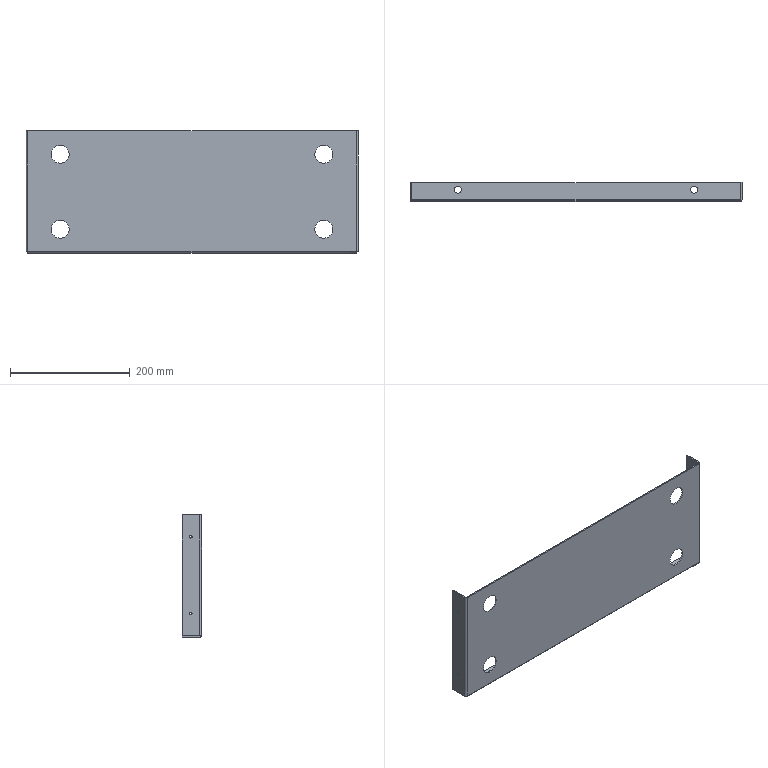Part | NX | 1 solid | 40 faces | box 554 x 32 x 204 mm | volume 275218 mm3 | plane 20 | cylinder 16 | spline 4 | commonest cylinder face diameters 4.2 x4 30 x4 2 x3 6 x3 12 x2
STEP:
#1=CARTESIAN_POINT('',(-274.293,30.,-103.));
#2=VERTEX_POINT('',#1);
#3=CARTESIAN_POINT('',(-274.293,1.,-103.));
#4=VERTEX_POINT('',#3);
#5=CARTESIAN_POINT('',(-274.293,0.,-103.));
#6=DIRECTION('',(0.,-1.,0.));
#7=VECTOR('',#6,1000.);
#8=LINE('',#5,#7);
#9=EDGE_CURVE('',#2,#4,#8,.T.);
#10=ORIENTED_EDGE('',*,*,#9,.F.);
#11=CARTESIAN_POINT('',(274.293,30.,-103.));
#12=VERTEX_POINT('',#11);
#13=CARTESIAN_POINT('',(-275.,30.,-103.));
#14=DIRECTION('',(1.,0.,0.));
#15=VECTOR('',#14,1000.);
#16=LINE('',#13,#15);
#17=EDGE_CURVE('',#2,#12,#16,.T.);
#18=ORIENTED_EDGE('',*,*,#17,.T.);
#19=CARTESIAN_POINT('',(274.293,1.,-103.));
#20=VERTEX_POINT('',#19);
#21=CARTESIAN_POINT('',(274.293,0.,-103.));
#22=DIRECTION('',(0.,-1.,0.));
#23=VECTOR('',#22,1000.);
#24=LINE('',#21,#23);
#25=EDGE_CURVE('',#12,#20,#24,.T.);
#26=ORIENTED_EDGE('',*,*,#25,.T.);
#27=CARTESIAN_POINT('',(0.,1.,-103.));
#28=DIRECTION('',(-1.,0.,0.));
#29=VECTOR('',#28,1000.);
#30=LINE('',#27,#29);
#31=EDGE_CURVE('',#20,#4,#30,.T.);
#32=ORIENTED_EDGE('',*,*,#31,.T.);
#33=EDGE_LOOP('',(#10,#18,#26,#32));
#34=FACE_BOUND('',#33,.T.);
#35=CARTESIAN_POINT('',(-197.,24.,-103.));
#36=VERTEX_POINT('',#35);
#37=CARTESIAN_POINT('',(-197.,18.,-103.));
#38=DIRECTION('',(0.,0.,-1.));
#39=DIRECTION('',(0.,1.,0.));
#40=AXIS2_PLACEMENT_3D('',#37,#38,#39);
#41=CIRCLE('',#40,6.);
#42=EDGE_CURVE('',#36,#36,#41,.T.);
#43=ORIENTED_EDGE('',*,*,#42,.F.);
#44=EDGE_LOOP('',(#43));
#45=FACE_BOUND('',#44,.T.);
#46=CARTESIAN_POINT('',(197.,24.,-103.));
#47=VERTEX_POINT('',#46);
#48=CARTESIAN_POINT('',(197.,18.,-103.));
#49=DIRECTION('',(0.,0.,1.));
#50=DIRECTION('',(0.,1.,0.));
#51=AXIS2_PLACEMENT_3D('',#48,#49,#50);
#52=CIRCLE('',#51,6.);
#53=EDGE_CURVE('',#47,#47,#52,.T.);
#54=ORIENTED_EDGE('',*,*,#53,.T.);
#55=EDGE_LOOP('',(#54));
#56=FACE_BOUND('',#55,.T.);
#57=CARTESIAN_POINT('',(0.,0.,-103.));
#58=DIRECTION('',(0.,0.,-1.));
#59=DIRECTION('',(0.,1.,0.));
#60=AXIS2_PLACEMENT_3D('',#57,#58,#59);
#61=PLANE('',#60);
#62=ADVANCED_FACE('',(#34,#45,#56),#61,.T.);
#63=CARTESIAN_POINT('',(-274.293,30.,-101.));
#64=VERTEX_POINT('',#63);
#65=CARTESIAN_POINT('',(274.293,30.,-101.));
#66=VERTEX_POINT('',#65);
#67=CARTESIAN_POINT('',(-275.,30.,-101.));
#68=DIRECTION('',(1.,0.,0.));
#69=VECTOR('',#68,1000.);
#70=LINE('',#67,#69);
#71=EDGE_CURVE('',#64,#66,#70,.T.);
#72=ORIENTED_EDGE('',*,*,#71,.F.);
#73=CARTESIAN_POINT('',(-274.293,1.,-101.));
#74=VERTEX_POINT('',#73);
#75=CARTESIAN_POINT('',(-274.293,0.,-101.));
#76=DIRECTION('',(0.,1.,0.));
#77=VECTOR('',#76,1000.);
#78=LINE('',#75,#77);
#79=EDGE_CURVE('',#74,#64,#78,.T.);
#80=ORIENTED_EDGE('',*,*,#79,.F.);
#81=CARTESIAN_POINT('',(274.293,1.,-101.));
#82=VERTEX_POINT('',#81);
#83=CARTESIAN_POINT('',(275.,1.,-101.));
#84=DIRECTION('',(-1.,0.,0.));
#85=VECTOR('',#84,1000.);
#86=LINE('',#83,#85);
#87=EDGE_CURVE('',#82,#74,#86,.T.);
#88=ORIENTED_EDGE('',*,*,#87,.F.);
#89=CARTESIAN_POINT('',(274.293,0.,-101.));
#90=DIRECTION('',(0.,1.,0.));
#91=VECTOR('',#90,1000.);
#92=LINE('',#89,#91);
#93=EDGE_CURVE('',#82,#66,#92,.T.);
#94=ORIENTED_EDGE('',*,*,#93,.T.);
#95=EDGE_LOOP('',(#72,#80,#88,#94));
#96=FACE_BOUND('',#95,.T.);
#97=CARTESIAN_POINT('',(-197.,24.,-101.));
#98=VERTEX_POINT('',#97);
#99=CARTESIAN_POINT('',(-197.,18.,-101.));
#100=DIRECTION('',(0.,0.,-1.));
#101=DIRECTION('',(0.,1.,0.));
#102=AXIS2_PLACEMENT_3D('',#99,#100,#101);
#103=CIRCLE('',#102,6.);
#104=EDGE_CURVE('',#98,#98,#103,.F.);
#105=ORIENTED_EDGE('',*,*,#104,.F.);
#106=EDGE_LOOP('',(#105));
#107=FACE_BOUND('',#106,.T.);
#108=CARTESIAN_POINT('',(197.,24.,-101.));
#109=VERTEX_POINT('',#108);
#110=CARTESIAN_POINT('',(197.,18.,-101.));
#111=DIRECTION('',(0.,0.,-1.));
#112=DIRECTION('',(0.,1.,0.));
#113=AXIS2_PLACEMENT_3D('',#110,#111,#112);
#114=CIRCLE('',#113,6.);
#115=EDGE_CURVE('',#109,#109,#114,.T.);
#116=ORIENTED_EDGE('',*,*,#115,.T.);
#117=EDGE_LOOP('',(#116));
#118=FACE_BOUND('',#117,.T.);
#119=CARTESIAN_POINT('',(0.,0.,-101.));
#120=DIRECTION('',(0.,0.,-1.));
#121=DIRECTION('',(0.,1.,0.));
#122=AXIS2_PLACEMENT_3D('',#119,#120,#121);
#123=PLANE('',#122);
#124=ADVANCED_FACE('',(#96,#107,#118),#123,.F.);
#125=CARTESIAN_POINT('',(220.,-2.,-48.));
#126=VERTEX_POINT('',#125);
#127=CARTESIAN_POINT('',(220.,-2.,-63.));
#128=DIRECTION('',(0.,-1.,0.));
#129=DIRECTION('',(0.,0.,1.));
#130=AXIS2_PLACEMENT_3D('',#127,#128,#129);
#131=CIRCLE('',#130,15.);
#132=EDGE_CURVE('',#126,#126,#131,.T.);
#133=ORIENTED_EDGE('',*,*,#132,.F.);
#134=EDGE_LOOP('',(#133));
#135=FACE_BOUND('',#134,.T.);
#136=CARTESIAN_POINT('',(-220.,-2.,47.));
#137=VERTEX_POINT('',#136);
#138=CARTESIAN_POINT('',(-220.,-2.,62.));
#139=DIRECTION('',(0.,-1.,0.));
#140=DIRECTION('',(0.,0.,-1.));
#141=AXIS2_PLACEMENT_3D('',#138,#139,#140);
#142=CIRCLE('',#141,15.);
#143=EDGE_CURVE('',#137,#137,#142,.T.);
#144=ORIENTED_EDGE('',*,*,#143,.F.);
#145=EDGE_LOOP('',(#144));
#146=FACE_BOUND('',#145,.T.);
#147=CARTESIAN_POINT('',(-220.,-2.,-78.));
#148=VERTEX_POINT('',#147);
#149=CARTESIAN_POINT('',(-220.,-2.,-63.));
#150=DIRECTION('',(0.,-1.,0.));
#151=DIRECTION('',(0.,0.,-1.));
#152=AXIS2_PLACEMENT_3D('',#149,#150,#151);
#153=CIRCLE('',#152,15.);
#154=EDGE_CURVE('',#148,#148,#153,.T.);
#155=ORIENTED_EDGE('',*,*,#154,.F.);
#156=EDGE_LOOP('',(#155));
#157=FACE_BOUND('',#156,.T.);
#158=CARTESIAN_POINT('',(-274.,-2.,101.));
#159=VERTEX_POINT('',#158);
#160=CARTESIAN_POINT('',(-274.,-2.,-100.));
#161=VERTEX_POINT('',#160);
#162=CARTESIAN_POINT('',(-274.,-2.,101.));
#163=DIRECTION('',(0.,0.,1.));
#164=VECTOR('',#163,1000.);
#165=LINE('',#162,#164);
#166=EDGE_CURVE('',#159,#161,#165,.F.);
#167=ORIENTED_EDGE('',*,*,#166,.T.);
#168=CARTESIAN_POINT('',(274.,-2.,-100.));
#169=VERTEX_POINT('',#168);
#170=CARTESIAN_POINT('',(-274.293,-2.,-100.));
#171=DIRECTION('',(-1.,0.,0.));
#172=VECTOR('',#171,1000.);
#173=LINE('',#170,#172);
#174=EDGE_CURVE('',#161,#169,#173,.F.);
#175=ORIENTED_EDGE('',*,*,#174,.T.);
#176=CARTESIAN_POINT('',(274.,-2.,101.));
#177=VERTEX_POINT('',#176);
#178=CARTESIAN_POINT('',(274.,-2.,-100.293));
#179=DIRECTION('',(0.,0.,-1.));
#180=VECTOR('',#179,1000.);
#181=LINE('',#178,#180);
#182=EDGE_CURVE('',#169,#177,#181,.F.);
#183=ORIENTED_EDGE('',*,*,#182,.T.);
#184=CARTESIAN_POINT('',(-275.,-2.,101.));
#185=DIRECTION('',(1.,0.,0.));
#186=VECTOR('',#185,1000.);
#187=LINE('',#184,#186);
#188=EDGE_CURVE('',#159,#177,#187,.T.);
#189=ORIENTED_EDGE('',*,*,#188,.F.);
#190=EDGE_LOOP('',(#167,#175,#183,#189));
#191=FACE_BOUND('',#190,.T.);
#192=CARTESIAN_POINT('',(220.,-2.,77.));
#193=VERTEX_POINT('',#192);
#194=CARTESIAN_POINT('',(220.,-2.,62.));
#195=DIRECTION('',(0.,-1.,0.));
#196=DIRECTION('',(0.,0.,1.));
#197=AXIS2_PLACEMENT_3D('',#194,#195,#196);
#198=CIRCLE('',#197,15.);
#199=EDGE_CURVE('',#193,#193,#198,.T.);
#200=ORIENTED_EDGE('',*,*,#199,.F.);
#201=EDGE_LOOP('',(#200));
#202=FACE_BOUND('',#201,.T.);
#203=CARTESIAN_POINT('',(0.,-2.,0.));
#204=DIRECTION('',(0.,-1.,0.));
#205=DIRECTION('',(0.,0.,-1.));
#206=AXIS2_PLACEMENT_3D('',#203,#204,#205);
#207=PLANE('',#206);
#208=ADVANCED_FACE('',(#135,#146,#157,#191,#202),#207,.T.);
#209=CARTESIAN_POINT('',(220.,0.,-48.));
#210=VERTEX_POINT('',#209);
#211=CARTESIAN_POINT('',(220.,0.,-63.));
#212=DIRECTION('',(0.,-1.,0.));
#213=DIRECTION('',(0.,0.,1.));
#214=AXIS2_PLACEMENT_3D('',#211,#212,#213);
#215=CIRCLE('',#214,15.);
#216=EDGE_CURVE('',#210,#210,#215,.T.);
#217=ORIENTED_EDGE('',*,*,#216,.T.);
#218=EDGE_LOOP('',(#217));
#219=FACE_BOUND('',#218,.T.);
#220=CARTESIAN_POINT('',(-220.,0.,77.));
#221=VERTEX_POINT('',#220);
#222=CARTESIAN_POINT('',(-220.,0.,62.));
#223=DIRECTION('',(0.,1.,0.));
#224=DIRECTION('',(0.,0.,1.));
#225=AXIS2_PLACEMENT_3D('',#222,#223,#224);
#226=CIRCLE('',#225,15.);
#227=EDGE_CURVE('',#221,#221,#226,.T.);
#228=ORIENTED_EDGE('',*,*,#227,.F.);
#229=EDGE_LOOP('',(#228));
#230=FACE_BOUND('',#229,.T.);
#231=CARTESIAN_POINT('',(-220.,0.,-48.));
#232=VERTEX_POINT('',#231);
#233=CARTESIAN_POINT('',(-220.,0.,-63.));
#234=DIRECTION('',(0.,1.,0.));
#235=DIRECTION('',(0.,0.,1.));
#236=AXIS2_PLACEMENT_3D('',#233,#234,#235);
#237=CIRCLE('',#236,15.);
#238=EDGE_CURVE('',#232,#232,#237,.T.);
#239=ORIENTED_EDGE('',*,*,#238,.F.);
#240=EDGE_LOOP('',(#239));
#241=FACE_BOUND('',#240,.T.);
#242=CARTESIAN_POINT('',(-274.,0.,-100.));
#243=VERTEX_POINT('',#242);
#244=CARTESIAN_POINT('',(274.,0.,-100.));
#245=VERTEX_POINT('',#244);
#246=CARTESIAN_POINT('',(-274.293,0.,-100.));
#247=DIRECTION('',(-1.,0.,0.));
#248=VECTOR('',#247,1000.);
#249=LINE('',#246,#248);
#250=EDGE_CURVE('',#243,#245,#249,.F.);
#251=ORIENTED_EDGE('',*,*,#250,.F.);
#252=CARTESIAN_POINT('',(-274.,0.,101.));
#253=VERTEX_POINT('',#252);
#254=CARTESIAN_POINT('',(-274.,0.,101.));
#255=DIRECTION('',(0.,0.,1.));
#256=VECTOR('',#255,1000.);
#257=LINE('',#254,#256);
#258=EDGE_CURVE('',#253,#243,#257,.F.);
#259=ORIENTED_EDGE('',*,*,#258,.F.);
#260=CARTESIAN_POINT('',(274.,0.,101.));
#261=VERTEX_POINT('',#260);
#262=CARTESIAN_POINT('',(-275.,0.,101.));
#263=DIRECTION('',(1.,0.,0.));
#264=VECTOR('',#263,1000.);
#265=LINE('',#262,#264);
#266=EDGE_CURVE('',#253,#261,#265,.T.);
#267=ORIENTED_EDGE('',*,*,#266,.T.);
#268=CARTESIAN_POINT('',(274.,0.,-100.293));
#269=DIRECTION('',(0.,0.,-1.));
#270=VECTOR('',#269,1000.);
#271=LINE('',#268,#270);
#272=EDGE_CURVE('',#245,#261,#271,.F.);
#273=ORIENTED_EDGE('',*,*,#272,.F.);
#274=EDGE_LOOP('',(#251,#259,#267,#273));
#275=FACE_BOUND('',#274,.T.);
#276=CARTESIAN_POINT('',(220.,0.,77.));
#277=VERTEX_POINT('',#276);
#278=CARTESIAN_POINT('',(220.,0.,62.));
#279=DIRECTION('',(0.,-1.,0.));
#280=DIRECTION('',(0.,0.,1.));
#281=AXIS2_PLACEMENT_3D('',#278,#279,#280);
#282=CIRCLE('',#281,15.);
#283=EDGE_CURVE('',#277,#277,#282,.T.);
#284=ORIENTED_EDGE('',*,*,#283,.T.);
#285=EDGE_LOOP('',(#284));
#286=FACE_BOUND('',#285,.T.);
#287=CARTESIAN_POINT('',(0.,0.,0.));
#288=DIRECTION('',(0.,-1.,0.));
#289=DIRECTION('',(0.,0.,-1.));
#290=AXIS2_PLACEMENT_3D('',#287,#288,#289);
#291=PLANE('',#290);
#292=ADVANCED_FACE('',(#219,#230,#241,#275,#286),#291,.F.);
#293=ORIENTED_EDGE('',*,*,#266,.F.);
#294=CARTESIAN_POINT('',(-274.,0.,101.));
#295=DIRECTION('',(0.,-1.,0.));
#296=VECTOR('',#295,1000.);
#297=LINE('',#294,#296);
#298=EDGE_CURVE('',#253,#159,#297,.T.);
#299=ORIENTED_EDGE('',*,*,#298,.T.);
#300=ORIENTED_EDGE('',*,*,#188,.T.);
#301=CARTESIAN_POINT('',(274.,0.,101.));
#302=DIRECTION('',(0.,-1.,0.));
#303=VECTOR('',#302,1000.);
#304=LINE('',#301,#303);
#305=EDGE_CURVE('',#261,#177,#304,.T.);
#306=ORIENTED_EDGE('',*,*,#305,.F.);
#307=EDGE_LOOP('',(#293,#299,#300,#306));
#308=FACE_BOUND('',#307,.T.);
#309=CARTESIAN_POINT('',(-275.,-2.,101.));
#310=DIRECTION('',(0.,0.,1.));
#311=DIRECTION('',(1.,0.,0.));
#312=AXIS2_PLACEMENT_3D('',#309,#310,#311);
#313=PLANE('',#312);
#314=ADVANCED_FACE('',(#308),#313,.T.);
#315=CARTESIAN_POINT('',(275.,1.,101.));
#316=VERTEX_POINT('',#315);
#317=CARTESIAN_POINT('',(277.,1.,101.));
#318=VERTEX_POINT('',#317);
#319=CARTESIAN_POINT('',(275.,1.,101.));
#320=DIRECTION('',(1.,0.,0.));
#321=VECTOR('',#320,1000.);
#322=LINE('',#319,#321);
#323=EDGE_CURVE('',#316,#318,#322,.T.);
#324=ORIENTED_EDGE('',*,*,#323,.F.);
#325=CARTESIAN_POINT('',(274.,1.,101.));
#326=DIRECTION('',(0.,0.,-1.));
#327=DIRECTION('',(-1.,0.,0.));
#328=AXIS2_PLACEMENT_3D('',#325,#326,#327);
#329=CIRCLE('',#328,1.);
#330=EDGE_CURVE('',#261,#316,#329,.F.);
#331=ORIENTED_EDGE('',*,*,#330,.F.);
#332=ORIENTED_EDGE('',*,*,#305,.T.);
#333=CARTESIAN_POINT('',(274.,1.,101.));
#334=DIRECTION('',(0.,0.,-1.));
#335=DIRECTION('',(-1.,0.,0.));
#336=AXIS2_PLACEMENT_3D('',#333,#334,#335);
#337=CIRCLE('',#336,3.);
#338=EDGE_CURVE('',#177,#318,#337,.F.);
#339=ORIENTED_EDGE('',*,*,#338,.T.);
#340=EDGE_LOOP('',(#324,#331,#332,#339));
#341=FACE_BOUND('',#340,.T.);
#342=CARTESIAN_POINT('',(274.,1.,101.));
#343=DIRECTION('',(0.,0.,1.));
#344=DIRECTION('',(1.,0.,0.));
#345=AXIS2_PLACEMENT_3D('',#342,#343,#344);
#346=PLANE('',#345);
#347=ADVANCED_FACE('',(#341),#346,.T.);
#348=CARTESIAN_POINT('',(275.,1.,-100.293));
#349=VERTEX_POINT('',#348);
#350=CARTESIAN_POINT('',(275.,1.,-100.293));
#351=CARTESIAN_POINT('',(275.,0.4764,-100.195));
#352=CARTESIAN_POINT('',(274.524,0.,-100.098));
#353=CARTESIAN_POINT('',(274.,0.,-100.));
#354=B_SPLINE_CURVE_WITH_KNOTS('',3,(#350,#351,#352,#353),.UNSPECIFIED.,.F.,.F.,(4,4),(0.,1.),.UNSPECIFIED.);
#355=EDGE_CURVE('',#349,#245,#354,.T.);
#356=ORIENTED_EDGE('',*,*,#355,.F.);
#357=CARTESIAN_POINT('',(277.,1.,-100.293));
#358=VERTEX_POINT('',#357);
#359=CARTESIAN_POINT('',(275.,1.,-100.293));
#360=DIRECTION('',(-1.,0.,0.));
#361=VECTOR('',#360,1000.);
#362=LINE('',#359,#361);
#363=EDGE_CURVE('',#358,#349,#362,.T.);
#364=ORIENTED_EDGE('',*,*,#363,.F.);
#365=CARTESIAN_POINT('',(277.,1.,-100.293));
#366=CARTESIAN_POINT('',(277.,0.2146,-100.244));
#367=CARTESIAN_POINT('',(276.35,-1.35,-100.146));
#368=CARTESIAN_POINT('',(274.785,-2.,-100.049));
#369=CARTESIAN_POINT('',(274.,-2.,-100.));
#370=B_SPLINE_CURVE_WITH_KNOTS('',3,(#365,#366,#367,#368,#369),.UNSPECIFIED.,.F.,.F.,(4,1,4),(0.,0.5,1.),.UNSPECIFIED.);
#371=EDGE_CURVE('',#358,#169,#370,.T.);
#372=ORIENTED_EDGE('',*,*,#371,.T.);
#373=CARTESIAN_POINT('',(274.,0.,-100.));
#374=DIRECTION('',(0.,-1.,0.));
#375=VECTOR('',#374,1000.);
#376=LINE('',#373,#375);
#377=EDGE_CURVE('',#245,#169,#376,.T.);
#378=ORIENTED_EDGE('',*,*,#377,.F.);
#379=EDGE_LOOP('',(#356,#364,#372,#378));
#380=FACE_BOUND('',#379,.T.);
#381=CARTESIAN_POINT('',(277.02,1.,-100.293));
#382=CARTESIAN_POINT('',(277.02,0.6046,-100.268));
#383=CARTESIAN_POINT('',(276.941,0.2095,-100.244));
#384=CARTESIAN_POINT('',(276.639,-0.5209,-100.195));
#385=CARTESIAN_POINT('',(276.415,-0.8559,-100.171));
#386=CARTESIAN_POINT('',(275.856,-1.415,-100.122));
#387=CARTESIAN_POINT('',(275.521,-1.639,-100.098));
#388=CARTESIAN_POINT('',(274.79,-1.941,-100.049));
#389=CARTESIAN_POINT('',(274.395,-2.02,-100.024));
#390=CARTESIAN_POINT('',(274.,-2.02,-100.));
#391=CARTESIAN_POINT('',(277.,1.,-100.293));
#392=CARTESIAN_POINT('',(277.,0.6072,-100.268));
#393=CARTESIAN_POINT('',(276.922,0.2148,-100.244));
#394=CARTESIAN_POINT('',(276.621,-0.5109,-100.195));
#395=CARTESIAN_POINT('',(276.399,-0.8436,-100.171));
#396=CARTESIAN_POINT('',(275.844,-1.399,-100.122));
#397=CARTESIAN_POINT('',(275.511,-1.621,-100.098));
#398=CARTESIAN_POINT('',(274.785,-1.922,-100.049));
#399=CARTESIAN_POINT('',(274.393,-2.,-100.024));
#400=CARTESIAN_POINT('',(274.,-2.,-100.));
#401=CARTESIAN_POINT('',(275.,1.,-100.293));
#402=CARTESIAN_POINT('',(275.,0.8691,-100.268));
#403=CARTESIAN_POINT('',(274.974,0.7383,-100.244));
#404=CARTESIAN_POINT('',(274.874,0.4964,-100.195));
#405=CARTESIAN_POINT('',(274.8,0.3855,-100.171));
#406=CARTESIAN_POINT('',(274.615,0.2003,-100.122));
#407=CARTESIAN_POINT('',(274.504,0.1262,-100.098));
#408=CARTESIAN_POINT('',(274.262,0.02603,-100.049));
#409=CARTESIAN_POINT('',(274.131,0.,-100.024));
#410=CARTESIAN_POINT('',(274.,0.,-100.));
#411=CARTESIAN_POINT('',(274.98,1.,-100.293));
#412=CARTESIAN_POINT('',(274.98,0.8717,-100.268));
#413=CARTESIAN_POINT('',(274.954,0.7435,-100.244));
#414=CARTESIAN_POINT('',(274.856,0.5066,-100.195));
#415=CARTESIAN_POINT('',(274.784,0.3979,-100.171));
#416=CARTESIAN_POINT('',(274.602,0.2165,-100.122));
#417=CARTESIAN_POINT('',(274.493,0.1439,-100.098));
#418=CARTESIAN_POINT('',(274.256,0.0457,-100.049));
#419=CARTESIAN_POINT('',(274.128,0.0202,-100.024));
#420=CARTESIAN_POINT('',(274.,0.0202,-100.));
#421=B_SPLINE_SURFACE_WITH_KNOTS('',1,3,((#381,#382,#383,#384,#385,#386,#387,#388,#389,#390),(#391,#392,#393,#394,#395,#396,#397,#398,#399,#400),(#401,#402,#403,#404,#405,#406,#407,#408,#409,#410),(#411,#412,#413,#414,#415,#416,#417,#418,#419,#420)),.RULED_SURF.,.F.,.F.,.F.,(2,1,1,2),(4,2,2,2,4),(-0.01,0.,1.,1.01),(0.,0.25,0.5,0.75,1.),.UNSPECIFIED.);
#422=ADVANCED_FACE('',(#380),#421,.F.);
#423=ORIENTED_EDGE('',*,*,#182,.F.);
#424=ORIENTED_EDGE('',*,*,#371,.F.);
#425=CARTESIAN_POINT('',(277.,1.,0.));
#426=DIRECTION('',(0.,0.,1.));
#427=VECTOR('',#426,1000.);
#428=LINE('',#425,#427);
#429=EDGE_CURVE('',#358,#318,#428,.T.);
#430=ORIENTED_EDGE('',*,*,#429,.T.);
#431=ORIENTED_EDGE('',*,*,#338,.F.);
#432=EDGE_LOOP('',(#423,#424,#430,#431));
#433=FACE_BOUND('',#432,.T.);
#434=CARTESIAN_POINT('',(274.,1.,-100.293));
#435=DIRECTION('',(0.,0.,-1.));
#436=DIRECTION('',(1.,0.,0.));
#437=AXIS2_PLACEMENT_3D('',#434,#435,#436);
#438=CYLINDRICAL_SURFACE('',#437,3.);
#439=ADVANCED_FACE('',(#433),#438,.T.);
#440=ORIENTED_EDGE('',*,*,#272,.T.);
#441=ORIENTED_EDGE('',*,*,#330,.T.);
#442=CARTESIAN_POINT('',(275.,1.,101.));
#443=DIRECTION('',(0.,0.,-1.));
#444=VECTOR('',#443,1000.);
#445=LINE('',#442,#444);
#446=EDGE_CURVE('',#316,#349,#445,.T.);
#447=ORIENTED_EDGE('',*,*,#446,.T.);
#448=ORIENTED_EDGE('',*,*,#355,.T.);
#449=EDGE_LOOP('',(#440,#441,#447,#448));
#450=FACE_BOUND('',#449,.T.);
#451=CARTESIAN_POINT('',(274.,1.,-100.293));
#452=DIRECTION('',(0.,0.,-1.));
#453=DIRECTION('',(1.,0.,0.));
#454=AXIS2_PLACEMENT_3D('',#451,#452,#453);
#455=CYLINDRICAL_SURFACE('',#454,1.);
#456=ADVANCED_FACE('',(#450),#455,.F.);
#457=ORIENTED_EDGE('',*,*,#323,.T.);
#458=CARTESIAN_POINT('',(277.,30.,101.));
#459=VERTEX_POINT('',#458);
#460=CARTESIAN_POINT('',(277.,0.,101.));
#461=DIRECTION('',(0.,-1.,0.));
#462=VECTOR('',#461,1000.);
#463=LINE('',#460,#462);
#464=EDGE_CURVE('',#459,#318,#463,.T.);
#465=ORIENTED_EDGE('',*,*,#464,.F.);
#466=CARTESIAN_POINT('',(275.,30.,101.));
#467=VERTEX_POINT('',#466);
#468=CARTESIAN_POINT('',(277.,30.,101.));
#469=DIRECTION('',(-1.,0.,0.));
#470=VECTOR('',#469,1000.);
#471=LINE('',#468,#470);
#472=EDGE_CURVE('',#459,#467,#471,.T.);
#473=ORIENTED_EDGE('',*,*,#472,.T.);
#474=CARTESIAN_POINT('',(275.,0.,101.));
#475=DIRECTION('',(0.,-1.,0.));
#476=VECTOR('',#475,1000.);
#477=LINE('',#474,#476);
#478=EDGE_CURVE('',#467,#316,#477,.T.);
#479=ORIENTED_EDGE('',*,*,#478,.T.);
#480=EDGE_LOOP('',(#457,#465,#473,#479));
#481=FACE_BOUND('',#480,.T.);
#482=CARTESIAN_POINT('',(277.,0.,101.));
#483=DIRECTION('',(0.,0.,-1.));
#484=DIRECTION('',(0.,1.,0.));
#485=AXIS2_PLACEMENT_3D('',#482,#483,#484);
#486=PLANE('',#485);
#487=ADVANCED_FACE('',(#481),#486,.F.);
#488=CARTESIAN_POINT('',(277.,13.9,64.5));
#489=VERTEX_POINT('',#488);
#490=CARTESIAN_POINT('',(277.,16.,64.5));
#491=DIRECTION('',(-1.,0.,0.));
#492=DIRECTION('',(0.,-1.,0.));
#493=AXIS2_PLACEMENT_3D('',#490,#491,#492);
#494=CIRCLE('',#493,2.1);
#495=EDGE_CURVE('',#489,#489,#494,.T.);
#496=ORIENTED_EDGE('',*,*,#495,.T.);
#497=EDGE_LOOP('',(#496));
#498=FACE_BOUND('',#497,.T.);
#499=CARTESIAN_POINT('',(277.,13.9,-63.5));
#500=VERTEX_POINT('',#499);
#501=CARTESIAN_POINT('',(277.,16.,-63.5));
#502=DIRECTION('',(-1.,0.,0.));
#503=DIRECTION('',(0.,-1.,0.));
#504=AXIS2_PLACEMENT_3D('',#501,#502,#503);
#505=CIRCLE('',#504,2.1);
#506=EDGE_CURVE('',#500,#500,#505,.T.);
#507=ORIENTED_EDGE('',*,*,#506,.T.);
#508=EDGE_LOOP('',(#507));
#509=FACE_BOUND('',#508,.T.);
#510=ORIENTED_EDGE('',*,*,#429,.F.);
#511=CARTESIAN_POINT('',(277.,30.,-100.293));
#512=VERTEX_POINT('',#511);
#513=CARTESIAN_POINT('',(277.,0.,-100.293));
#514=DIRECTION('',(0.,1.,0.));
#515=VECTOR('',#514,1000.);
#516=LINE('',#513,#515);
#517=EDGE_CURVE('',#358,#512,#516,.T.);
#518=ORIENTED_EDGE('',*,*,#517,.T.);
#519=CARTESIAN_POINT('',(277.,30.,101.));
#520=DIRECTION('',(0.,0.,1.));
#521=VECTOR('',#520,1000.);
#522=LINE('',#519,#521);
#523=EDGE_CURVE('',#512,#459,#522,.T.);
#524=ORIENTED_EDGE('',*,*,#523,.T.);
#525=ORIENTED_EDGE('',*,*,#464,.T.);
#526=EDGE_LOOP('',(#510,#518,#524,#525));
#527=FACE_BOUND('',#526,.T.);
#528=CARTESIAN_POINT('',(277.,0.,0.));
#529=DIRECTION('',(-1.,0.,0.));
#530=DIRECTION('',(0.,-1.,0.));
#531=AXIS2_PLACEMENT_3D('',#528,#529,#530);
#532=PLANE('',#531);
#533=ADVANCED_FACE('',(#498,#509,#527),#532,.F.);
#534=CARTESIAN_POINT('',(275.,13.9,64.5));
#535=VERTEX_POINT('',#534);
#536=CARTESIAN_POINT('',(275.,16.,64.5));
#537=DIRECTION('',(-1.,0.,0.));
#538=DIRECTION('',(0.,-1.,0.));
#539=AXIS2_PLACEMENT_3D('',#536,#537,#538);
#540=CIRCLE('',#539,2.1);
#541=EDGE_CURVE('',#535,#535,#540,.T.);
#542=ORIENTED_EDGE('',*,*,#541,.F.);
#543=EDGE_LOOP('',(#542));
#544=FACE_BOUND('',#543,.T.);
#545=CARTESIAN_POINT('',(275.,13.9,-63.5));
#546=VERTEX_POINT('',#545);
#547=CARTESIAN_POINT('',(275.,16.,-63.5));
#548=DIRECTION('',(-1.,0.,0.));
#549=DIRECTION('',(0.,-1.,0.));
#550=AXIS2_PLACEMENT_3D('',#547,#548,#549);
#551=CIRCLE('',#550,2.1);
#552=EDGE_CURVE('',#546,#546,#551,.T.);
#553=ORIENTED_EDGE('',*,*,#552,.F.);
#554=EDGE_LOOP('',(#553));
#555=FACE_BOUND('',#554,.T.);
#556=CARTESIAN_POINT('',(275.,30.,-100.293));
#557=VERTEX_POINT('',#556);
#558=CARTESIAN_POINT('',(275.,0.,-100.293));
#559=DIRECTION('',(0.,1.,0.));
#560=VECTOR('',#559,1000.);
#561=LINE('',#558,#560);
#562=EDGE_CURVE('',#349,#557,#561,.T.);
#563=ORIENTED_EDGE('',*,*,#562,.F.);
#564=ORIENTED_EDGE('',*,*,#446,.F.);
#565=ORIENTED_EDGE('',*,*,#478,.F.);
#566=CARTESIAN_POINT('',(275.,30.,101.));
#567=DIRECTION('',(0.,0.,1.));
#568=VECTOR('',#567,1000.);
#569=LINE('',#566,#568);
#570=EDGE_CURVE('',#557,#467,#569,.T.);
#571=ORIENTED_EDGE('',*,*,#570,.F.);
#572=EDGE_LOOP('',(#563,#564,#565,#571));
#573=FACE_BOUND('',#572,.T.);
#574=CARTESIAN_POINT('',(275.,0.,0.));
#575=DIRECTION('',(-1.,0.,0.));
#576=DIRECTION('',(0.,-1.,0.));
#577=AXIS2_PLACEMENT_3D('',#574,#575,#576);
#578=PLANE('',#577);
#579=ADVANCED_FACE('',(#544,#555,#573),#578,.T.);
#580=ORIENTED_EDGE('',*,*,#523,.F.);
#581=CARTESIAN_POINT('',(277.,30.,-100.293));
#582=DIRECTION('',(-1.,0.,0.));
#583=VECTOR('',#582,1000.);
#584=LINE('',#581,#583);
#585=EDGE_CURVE('',#512,#557,#584,.T.);
#586=ORIENTED_EDGE('',*,*,#585,.T.);
#587=ORIENTED_EDGE('',*,*,#570,.T.);
#588=ORIENTED_EDGE('',*,*,#472,.F.);
#589=EDGE_LOOP('',(#580,#586,#587,#588));
#590=FACE_BOUND('',#589,.T.);
#591=CARTESIAN_POINT('',(277.,30.,101.));
#592=DIRECTION('',(0.,-1.,0.));
#593=DIRECTION('',(1.,0.,0.));
#594=AXIS2_PLACEMENT_3D('',#591,#592,#593);
#595=PLANE('',#594);
#596=ADVANCED_FACE('',(#590),#595,.F.);
#597=ORIENTED_EDGE('',*,*,#585,.F.);
#598=ORIENTED_EDGE('',*,*,#517,.F.);
#599=ORIENTED_EDGE('',*,*,#363,.T.);
#600=ORIENTED_EDGE('',*,*,#562,.T.);
#601=EDGE_LOOP('',(#597,#598,#599,#600));
#602=FACE_BOUND('',#601,.T.);
#603=CARTESIAN_POINT('',(275.,0.,-100.293));
#604=DIRECTION('',(0.,0.,1.));
#605=DIRECTION('',(0.,-1.,0.));
#606=AXIS2_PLACEMENT_3D('',#603,#604,#605);
#607=PLANE('',#606);
#608=ADVANCED_FACE('',(#602),#607,.F.);
#609=CARTESIAN_POINT('',(-277.,1.,-100.293));
#610=VERTEX_POINT('',#609);
#611=CARTESIAN_POINT('',(-275.,1.,-100.293));
#612=VERTEX_POINT('',#611);
#613=CARTESIAN_POINT('',(-275.,1.,-100.293));
#614=DIRECTION('',(1.,0.,0.));
#615=VECTOR('',#614,1000.);
#616=LINE('',#613,#615);
#617=EDGE_CURVE('',#610,#612,#616,.T.);
#618=ORIENTED_EDGE('',*,*,#617,.T.);
#619=CARTESIAN_POINT('',(-274.,0.,-100.));
#620=CARTESIAN_POINT('',(-274.524,0.,-100.098));
#621=CARTESIAN_POINT('',(-275.,0.4764,-100.195));
#622=CARTESIAN_POINT('',(-275.,1.,-100.293));
#623=B_SPLINE_CURVE_WITH_KNOTS('',3,(#619,#620,#621,#622),.UNSPECIFIED.,.F.,.F.,(4,4),(0.,1.),.UNSPECIFIED.);
#624=EDGE_CURVE('',#243,#612,#623,.T.);
#625=ORIENTED_EDGE('',*,*,#624,.F.);
#626=CARTESIAN_POINT('',(-274.,0.,-100.));
#627=DIRECTION('',(0.,-1.,0.));
#628=VECTOR('',#627,1000.);
#629=LINE('',#626,#628);
#630=EDGE_CURVE('',#243,#161,#629,.T.);
#631=ORIENTED_EDGE('',*,*,#630,.T.);
#632=CARTESIAN_POINT('',(-274.,-2.,-100.));
#633=CARTESIAN_POINT('',(-274.785,-2.,-100.049));
#634=CARTESIAN_POINT('',(-276.35,-1.35,-100.146));
#635=CARTESIAN_POINT('',(-277.,0.2146,-100.244));
#636=CARTESIAN_POINT('',(-277.,1.,-100.293));
#637=B_SPLINE_CURVE_WITH_KNOTS('',3,(#632,#633,#634,#635,#636),.UNSPECIFIED.,.F.,.F.,(4,1,4),(0.,0.5,1.),.UNSPECIFIED.);
#638=EDGE_CURVE('',#161,#610,#637,.T.);
#639=ORIENTED_EDGE('',*,*,#638,.T.);
#640=EDGE_LOOP('',(#618,#625,#631,#639));
#641=FACE_BOUND('',#640,.T.);
#642=CARTESIAN_POINT('',(-274.,-2.02,-100.));
#643=CARTESIAN_POINT('',(-274.395,-2.02,-100.024));
#644=CARTESIAN_POINT('',(-274.79,-1.941,-100.049));
#645=CARTESIAN_POINT('',(-275.521,-1.639,-100.098));
#646=CARTESIAN_POINT('',(-275.856,-1.415,-100.122));
#647=CARTESIAN_POINT('',(-276.415,-0.8559,-100.171));
#648=CARTESIAN_POINT('',(-276.639,-0.5209,-100.195));
#649=CARTESIAN_POINT('',(-276.941,0.2095,-100.244));
#650=CARTESIAN_POINT('',(-277.02,0.6046,-100.268));
#651=CARTESIAN_POINT('',(-277.02,1.,-100.293));
#652=CARTESIAN_POINT('',(-274.,-2.,-100.));
#653=CARTESIAN_POINT('',(-274.393,-2.,-100.024));
#654=CARTESIAN_POINT('',(-274.785,-1.922,-100.049));
#655=CARTESIAN_POINT('',(-275.511,-1.621,-100.098));
#656=CARTESIAN_POINT('',(-275.844,-1.399,-100.122));
#657=CARTESIAN_POINT('',(-276.399,-0.8436,-100.171));
#658=CARTESIAN_POINT('',(-276.621,-0.5109,-100.195));
#659=CARTESIAN_POINT('',(-276.922,0.2148,-100.244));
#660=CARTESIAN_POINT('',(-277.,0.6072,-100.268));
#661=CARTESIAN_POINT('',(-277.,1.,-100.293));
#662=CARTESIAN_POINT('',(-274.,0.,-100.));
#663=CARTESIAN_POINT('',(-274.131,0.,-100.024));
#664=CARTESIAN_POINT('',(-274.262,0.02603,-100.049));
#665=CARTESIAN_POINT('',(-274.504,0.1262,-100.098));
#666=CARTESIAN_POINT('',(-274.615,0.2003,-100.122));
#667=CARTESIAN_POINT('',(-274.8,0.3855,-100.171));
#668=CARTESIAN_POINT('',(-274.874,0.4964,-100.195));
#669=CARTESIAN_POINT('',(-274.974,0.7383,-100.244));
#670=CARTESIAN_POINT('',(-275.,0.8691,-100.268));
#671=CARTESIAN_POINT('',(-275.,1.,-100.293));
#672=CARTESIAN_POINT('',(-274.,0.0202,-100.));
#673=CARTESIAN_POINT('',(-274.128,0.0202,-100.024));
#674=CARTESIAN_POINT('',(-274.256,0.0457,-100.049));
#675=CARTESIAN_POINT('',(-274.493,0.1439,-100.098));
#676=CARTESIAN_POINT('',(-274.602,0.2165,-100.122));
#677=CARTESIAN_POINT('',(-274.784,0.3979,-100.171));
#678=CARTESIAN_POINT('',(-274.856,0.5066,-100.195));
#679=CARTESIAN_POINT('',(-274.954,0.7435,-100.244));
#680=CARTESIAN_POINT('',(-274.98,0.8717,-100.268));
#681=CARTESIAN_POINT('',(-274.98,1.,-100.293));
#682=B_SPLINE_SURFACE_WITH_KNOTS('',1,3,((#642,#643,#644,#645,#646,#647,#648,#649,#650,#651),(#652,#653,#654,#655,#656,#657,#658,#659,#660,#661),(#662,#663,#664,#665,#666,#667,#668,#669,#670,#671),(#672,#673,#674,#675,#676,#677,#678,#679,#680,#681)),.RULED_SURF.,.F.,.F.,.F.,(2,1,1,2),(4,2,2,2,4),(-0.01,0.,1.,1.01),(0.,0.25,0.5,0.75,1.),.UNSPECIFIED.);
#683=ADVANCED_FACE('',(#641),#682,.F.);
#684=CARTESIAN_POINT('',(-275.,1.,101.));
#685=VERTEX_POINT('',#684);
#686=CARTESIAN_POINT('',(-274.,1.,101.));
#687=DIRECTION('',(0.,0.,1.));
#688=DIRECTION('',(1.,0.,0.));
#689=AXIS2_PLACEMENT_3D('',#686,#687,#688);
#690=CIRCLE('',#689,1.);
#691=EDGE_CURVE('',#685,#253,#690,.T.);
#692=ORIENTED_EDGE('',*,*,#691,.F.);
#693=CARTESIAN_POINT('',(-277.,1.,101.));
#694=VERTEX_POINT('',#693);
#695=CARTESIAN_POINT('',(-275.,1.,101.));
#696=DIRECTION('',(-1.,0.,0.));
#697=VECTOR('',#696,1000.);
#698=LINE('',#695,#697);
#699=EDGE_CURVE('',#685,#694,#698,.T.);
#700=ORIENTED_EDGE('',*,*,#699,.T.);
#701=CARTESIAN_POINT('',(-274.,1.,101.));
#702=DIRECTION('',(0.,0.,1.));
#703=DIRECTION('',(1.,0.,0.));
#704=AXIS2_PLACEMENT_3D('',#701,#702,#703);
#705=CIRCLE('',#704,3.);
#706=EDGE_CURVE('',#694,#159,#705,.T.);
#707=ORIENTED_EDGE('',*,*,#706,.T.);
#708=ORIENTED_EDGE('',*,*,#298,.F.);
#709=EDGE_LOOP('',(#692,#700,#707,#708));
#710=FACE_BOUND('',#709,.T.);
#711=CARTESIAN_POINT('',(-274.,1.,101.));
#712=DIRECTION('',(0.,0.,-1.));
#713=DIRECTION('',(-1.,0.,0.));
#714=AXIS2_PLACEMENT_3D('',#711,#712,#713);
#715=PLANE('',#714);
#716=ADVANCED_FACE('',(#710),#715,.F.);
#717=ORIENTED_EDGE('',*,*,#166,.F.);
#718=ORIENTED_EDGE('',*,*,#706,.F.);
#719=CARTESIAN_POINT('',(-277.,1.,0.));
#720=DIRECTION('',(0.,0.,1.));
#721=VECTOR('',#720,1000.);
#722=LINE('',#719,#721);
#723=EDGE_CURVE('',#610,#694,#722,.T.);
#724=ORIENTED_EDGE('',*,*,#723,.F.);
#725=ORIENTED_EDGE('',*,*,#638,.F.);
#726=EDGE_LOOP('',(#717,#718,#724,#725));
#727=FACE_BOUND('',#726,.T.);
#728=CARTESIAN_POINT('',(-274.,1.,101.));
#729=DIRECTION('',(0.,0.,1.));
#730=DIRECTION('',(-1.,0.,0.));
#731=AXIS2_PLACEMENT_3D('',#728,#729,#730);
#732=CYLINDRICAL_SURFACE('',#731,3.);
#733=ADVANCED_FACE('',(#727),#732,.T.);
#734=ORIENTED_EDGE('',*,*,#258,.T.);
#735=ORIENTED_EDGE('',*,*,#624,.T.);
#736=CARTESIAN_POINT('',(-275.,1.,-101.));
#737=DIRECTION('',(0.,0.,1.));
#738=VECTOR('',#737,1000.);
#739=LINE('',#736,#738);
#740=EDGE_CURVE('',#612,#685,#739,.T.);
#741=ORIENTED_EDGE('',*,*,#740,.T.);
#742=ORIENTED_EDGE('',*,*,#691,.T.);
#743=EDGE_LOOP('',(#734,#735,#741,#742));
#744=FACE_BOUND('',#743,.T.);
#745=CARTESIAN_POINT('',(-274.,1.,101.));
#746=DIRECTION('',(0.,0.,1.));
#747=DIRECTION('',(-1.,0.,0.));
#748=AXIS2_PLACEMENT_3D('',#745,#746,#747);
#749=CYLINDRICAL_SURFACE('',#748,1.);
#750=ADVANCED_FACE('',(#744),#749,.F.);
#751=CARTESIAN_POINT('',(-277.,30.,-100.293));
#752=VERTEX_POINT('',#751);
#753=CARTESIAN_POINT('',(-277.,0.,-100.293));
#754=DIRECTION('',(0.,-1.,0.));
#755=VECTOR('',#754,1000.);
#756=LINE('',#753,#755);
#757=EDGE_CURVE('',#752,#610,#756,.T.);
#758=ORIENTED_EDGE('',*,*,#757,.F.);
#759=CARTESIAN_POINT('',(-275.,30.,-100.293));
#760=VERTEX_POINT('',#759);
#761=CARTESIAN_POINT('',(-277.,30.,-100.293));
#762=DIRECTION('',(1.,0.,0.));
#763=VECTOR('',#762,1000.);
#764=LINE('',#761,#763);
#765=EDGE_CURVE('',#752,#760,#764,.T.);
#766=ORIENTED_EDGE('',*,*,#765,.T.);
#767=CARTESIAN_POINT('',(-275.,0.,-100.293));
#768=DIRECTION('',(0.,1.,0.));
#769=VECTOR('',#768,1000.);
#770=LINE('',#767,#769);
#771=EDGE_CURVE('',#612,#760,#770,.T.);
#772=ORIENTED_EDGE('',*,*,#771,.F.);
#773=ORIENTED_EDGE('',*,*,#617,.F.);
#774=EDGE_LOOP('',(#758,#766,#772,#773));
#775=FACE_BOUND('',#774,.T.);
#776=CARTESIAN_POINT('',(-275.,0.,-100.293));
#777=DIRECTION('',(0.,0.,-1.));
#778=DIRECTION('',(0.,1.,0.));
#779=AXIS2_PLACEMENT_3D('',#776,#777,#778);
#780=PLANE('',#779);
#781=ADVANCED_FACE('',(#775),#780,.T.);
#782=CARTESIAN_POINT('',(-277.,16.,66.6));
#783=VERTEX_POINT('',#782);
#784=CARTESIAN_POINT('',(-277.,16.,64.5));
#785=DIRECTION('',(-1.,0.,0.));
#786=DIRECTION('',(0.,0.,1.));
#787=AXIS2_PLACEMENT_3D('',#784,#785,#786);
#788=CIRCLE('',#787,2.1);
#789=EDGE_CURVE('',#783,#783,#788,.T.);
#790=ORIENTED_EDGE('',*,*,#789,.F.);
#791=EDGE_LOOP('',(#790));
#792=FACE_BOUND('',#791,.T.);
#793=CARTESIAN_POINT('',(-277.,16.,-61.4));
#794=VERTEX_POINT('',#793);
#795=CARTESIAN_POINT('',(-277.,16.,-63.5));
#796=DIRECTION('',(-1.,0.,0.));
#797=DIRECTION('',(0.,0.,1.));
#798=AXIS2_PLACEMENT_3D('',#795,#796,#797);
#799=CIRCLE('',#798,2.1);
#800=EDGE_CURVE('',#794,#794,#799,.T.);
#801=ORIENTED_EDGE('',*,*,#800,.F.);
#802=EDGE_LOOP('',(#801));
#803=FACE_BOUND('',#802,.T.);
#804=CARTESIAN_POINT('',(-277.,30.,101.));
#805=VERTEX_POINT('',#804);
#806=CARTESIAN_POINT('',(-277.,30.,101.));
#807=DIRECTION('',(0.,0.,-1.));
#808=VECTOR('',#807,1000.);
#809=LINE('',#806,#808);
#810=EDGE_CURVE('',#805,#752,#809,.T.);
#811=ORIENTED_EDGE('',*,*,#810,.T.);
#812=ORIENTED_EDGE('',*,*,#757,.T.);
#813=ORIENTED_EDGE('',*,*,#723,.T.);
#814=CARTESIAN_POINT('',(-277.,0.,101.));
#815=DIRECTION('',(0.,1.,0.));
#816=VECTOR('',#815,1000.);
#817=LINE('',#814,#816);
#818=EDGE_CURVE('',#694,#805,#817,.T.);
#819=ORIENTED_EDGE('',*,*,#818,.T.);
#820=EDGE_LOOP('',(#811,#812,#813,#819));
#821=FACE_BOUND('',#820,.T.);
#822=CARTESIAN_POINT('',(-277.,0.,0.));
#823=DIRECTION('',(-1.,0.,0.));
#824=DIRECTION('',(0.,-1.,0.));
#825=AXIS2_PLACEMENT_3D('',#822,#823,#824);
#826=PLANE('',#825);
#827=ADVANCED_FACE('',(#792,#803,#821),#826,.T.);
#828=CARTESIAN_POINT('',(-275.,13.9,64.5));
#829=VERTEX_POINT('',#828);
#830=CARTESIAN_POINT('',(-275.,16.,64.5));
#831=DIRECTION('',(-1.,0.,0.));
#832=DIRECTION('',(0.,-1.,0.));
#833=AXIS2_PLACEMENT_3D('',#830,#831,#832);
#834=CIRCLE('',#833,2.1);
#835=EDGE_CURVE('',#829,#829,#834,.T.);
#836=ORIENTED_EDGE('',*,*,#835,.T.);
#837=EDGE_LOOP('',(#836));
#838=FACE_BOUND('',#837,.T.);
#839=CARTESIAN_POINT('',(-275.,13.9,-63.5));
#840=VERTEX_POINT('',#839);
#841=CARTESIAN_POINT('',(-275.,16.,-63.5));
#842=DIRECTION('',(-1.,0.,0.));
#843=DIRECTION('',(0.,-1.,0.));
#844=AXIS2_PLACEMENT_3D('',#841,#842,#843);
#845=CIRCLE('',#844,2.1);
#846=EDGE_CURVE('',#840,#840,#845,.T.);
#847=ORIENTED_EDGE('',*,*,#846,.T.);
#848=EDGE_LOOP('',(#847));
#849=FACE_BOUND('',#848,.T.);
#850=ORIENTED_EDGE('',*,*,#771,.T.);
#851=CARTESIAN_POINT('',(-275.,30.,101.));
#852=VERTEX_POINT('',#851);
#853=CARTESIAN_POINT('',(-275.,30.,101.));
#854=DIRECTION('',(0.,0.,-1.));
#855=VECTOR('',#854,1000.);
#856=LINE('',#853,#855);
#857=EDGE_CURVE('',#852,#760,#856,.T.);
#858=ORIENTED_EDGE('',*,*,#857,.F.);
#859=CARTESIAN_POINT('',(-275.,0.,101.));
#860=DIRECTION('',(0.,1.,0.));
#861=VECTOR('',#860,1000.);
#862=LINE('',#859,#861);
#863=EDGE_CURVE('',#685,#852,#862,.T.);
#864=ORIENTED_EDGE('',*,*,#863,.F.);
#865=ORIENTED_EDGE('',*,*,#740,.F.);
#866=EDGE_LOOP('',(#850,#858,#864,#865));
#867=FACE_BOUND('',#866,.T.);
#868=CARTESIAN_POINT('',(-275.,0.,0.));
#869=DIRECTION('',(-1.,0.,0.));
#870=DIRECTION('',(0.,-1.,0.));
#871=AXIS2_PLACEMENT_3D('',#868,#869,#870);
#872=PLANE('',#871);
#873=ADVANCED_FACE('',(#838,#849,#867),#872,.F.);
#874=ORIENTED_EDGE('',*,*,#765,.F.);
#875=ORIENTED_EDGE('',*,*,#810,.F.);
#876=CARTESIAN_POINT('',(-277.,30.,101.));
#877=DIRECTION('',(1.,0.,0.));
#878=VECTOR('',#877,1000.);
#879=LINE('',#876,#878);
#880=EDGE_CURVE('',#805,#852,#879,.T.);
#881=ORIENTED_EDGE('',*,*,#880,.T.);
#882=ORIENTED_EDGE('',*,*,#857,.T.);
#883=EDGE_LOOP('',(#874,#875,#881,#882));
#884=FACE_BOUND('',#883,.T.);
#885=CARTESIAN_POINT('',(-277.,30.,101.));
#886=DIRECTION('',(0.,-1.,0.));
#887=DIRECTION('',(1.,0.,0.));
#888=AXIS2_PLACEMENT_3D('',#885,#886,#887);
#889=PLANE('',#888);
#890=ADVANCED_FACE('',(#884),#889,.F.);
#891=ORIENTED_EDGE('',*,*,#699,.F.);
#892=ORIENTED_EDGE('',*,*,#863,.T.);
#893=ORIENTED_EDGE('',*,*,#880,.F.);
#894=ORIENTED_EDGE('',*,*,#818,.F.);
#895=EDGE_LOOP('',(#891,#892,#893,#894));
#896=FACE_BOUND('',#895,.T.);
#897=CARTESIAN_POINT('',(-277.,0.,101.));
#898=DIRECTION('',(0.,0.,-1.));
#899=DIRECTION('',(0.,1.,0.));
#900=AXIS2_PLACEMENT_3D('',#897,#898,#899);
#901=PLANE('',#900);
#902=ADVANCED_FACE('',(#896),#901,.F.);
#903=CARTESIAN_POINT('',(274.293,1.,-101.));
#904=DIRECTION('',(0.,0.,1.));
#905=VECTOR('',#904,1000.);
#906=LINE('',#903,#905);
#907=EDGE_CURVE('',#20,#82,#906,.T.);
#908=ORIENTED_EDGE('',*,*,#907,.T.);
#909=CARTESIAN_POINT('',(274.,0.,-100.));
#910=CARTESIAN_POINT('',(274.098,0.,-100.524));
#911=CARTESIAN_POINT('',(274.195,0.4764,-101.));
#912=CARTESIAN_POINT('',(274.293,1.,-101.));
#913=B_SPLINE_CURVE_WITH_KNOTS('',3,(#909,#910,#911,#912),.UNSPECIFIED.,.F.,.F.,(4,4),(0.,1.),.UNSPECIFIED.);
#914=EDGE_CURVE('',#245,#82,#913,.T.);
#915=ORIENTED_EDGE('',*,*,#914,.F.);
#916=ORIENTED_EDGE('',*,*,#377,.T.);
#917=CARTESIAN_POINT('',(274.,-2.,-100.));
#918=CARTESIAN_POINT('',(274.049,-2.,-100.785));
#919=CARTESIAN_POINT('',(274.146,-1.35,-102.35));
#920=CARTESIAN_POINT('',(274.244,0.2146,-103.));
#921=CARTESIAN_POINT('',(274.293,1.,-103.));
#922=B_SPLINE_CURVE_WITH_KNOTS('',3,(#917,#918,#919,#920,#921),.UNSPECIFIED.,.F.,.F.,(4,1,4),(0.,0.5,1.),.UNSPECIFIED.);
#923=EDGE_CURVE('',#169,#20,#922,.T.);
#924=ORIENTED_EDGE('',*,*,#923,.T.);
#925=EDGE_LOOP('',(#908,#915,#916,#924));
#926=FACE_BOUND('',#925,.T.);
#927=CARTESIAN_POINT('',(274.,-2.02,-100.));
#928=CARTESIAN_POINT('',(274.024,-2.02,-100.395));
#929=CARTESIAN_POINT('',(274.049,-1.941,-100.79));
#930=CARTESIAN_POINT('',(274.098,-1.639,-101.521));
#931=CARTESIAN_POINT('',(274.122,-1.415,-101.856));
#932=CARTESIAN_POINT('',(274.171,-0.8559,-102.415));
#933=CARTESIAN_POINT('',(274.195,-0.5209,-102.639));
#934=CARTESIAN_POINT('',(274.244,0.2095,-102.941));
#935=CARTESIAN_POINT('',(274.268,0.6046,-103.02));
#936=CARTESIAN_POINT('',(274.293,1.,-103.02));
#937=CARTESIAN_POINT('',(274.,-2.,-100.));
#938=CARTESIAN_POINT('',(274.024,-2.,-100.393));
#939=CARTESIAN_POINT('',(274.049,-1.922,-100.785));
#940=CARTESIAN_POINT('',(274.098,-1.621,-101.511));
#941=CARTESIAN_POINT('',(274.122,-1.399,-101.844));
#942=CARTESIAN_POINT('',(274.171,-0.8436,-102.399));
#943=CARTESIAN_POINT('',(274.195,-0.5109,-102.621));
#944=CARTESIAN_POINT('',(274.244,0.2148,-102.922));
#945=CARTESIAN_POINT('',(274.268,0.6072,-103.));
#946=CARTESIAN_POINT('',(274.293,1.,-103.));
#947=CARTESIAN_POINT('',(274.,0.,-100.));
#948=CARTESIAN_POINT('',(274.024,0.,-100.131));
#949=CARTESIAN_POINT('',(274.049,0.02603,-100.262));
#950=CARTESIAN_POINT('',(274.098,0.1262,-100.504));
#951=CARTESIAN_POINT('',(274.122,0.2003,-100.615));
#952=CARTESIAN_POINT('',(274.171,0.3855,-100.8));
#953=CARTESIAN_POINT('',(274.195,0.4964,-100.874));
#954=CARTESIAN_POINT('',(274.244,0.7383,-100.974));
#955=CARTESIAN_POINT('',(274.268,0.8691,-101.));
#956=CARTESIAN_POINT('',(274.293,1.,-101.));
#957=CARTESIAN_POINT('',(274.,0.0202,-100.));
#958=CARTESIAN_POINT('',(274.024,0.0202,-100.128));
#959=CARTESIAN_POINT('',(274.049,0.0457,-100.256));
#960=CARTESIAN_POINT('',(274.098,0.1439,-100.493));
#961=CARTESIAN_POINT('',(274.122,0.2165,-100.602));
#962=CARTESIAN_POINT('',(274.171,0.3979,-100.784));
#963=CARTESIAN_POINT('',(274.195,0.5066,-100.856));
#964=CARTESIAN_POINT('',(274.244,0.7435,-100.954));
#965=CARTESIAN_POINT('',(274.268,0.8717,-100.98));
#966=CARTESIAN_POINT('',(274.293,1.,-100.98));
#967=B_SPLINE_SURFACE_WITH_KNOTS('',1,3,((#927,#928,#929,#930,#931,#932,#933,#934,#935,#936),(#937,#938,#939,#940,#941,#942,#943,#944,#945,#946),(#947,#948,#949,#950,#951,#952,#953,#954,#955,#956),(#957,#958,#959,#960,#961,#962,#963,#964,#965,#966)),.RULED_SURF.,.F.,.F.,.F.,(2,1,1,2),(4,2,2,2,4),(-0.01,0.,1.,1.01),(0.,0.25,0.5,0.75,1.),.UNSPECIFIED.);
#968=ADVANCED_FACE('',(#926),#967,.F.);
#969=CARTESIAN_POINT('',(-274.293,1.,-101.));
#970=CARTESIAN_POINT('',(-274.195,0.4764,-101.));
#971=CARTESIAN_POINT('',(-274.098,0.,-100.524));
#972=CARTESIAN_POINT('',(-274.,0.,-100.));
#973=B_SPLINE_CURVE_WITH_KNOTS('',3,(#969,#970,#971,#972),.UNSPECIFIED.,.F.,.F.,(4,4),(0.,1.),.UNSPECIFIED.);
#974=EDGE_CURVE('',#74,#243,#973,.T.);
#975=ORIENTED_EDGE('',*,*,#974,.F.);
#976=CARTESIAN_POINT('',(-274.293,1.,-101.));
#977=DIRECTION('',(0.,0.,1.));
#978=VECTOR('',#977,1000.);
#979=LINE('',#976,#978);
#980=EDGE_CURVE('',#4,#74,#979,.T.);
#981=ORIENTED_EDGE('',*,*,#980,.F.);
#982=CARTESIAN_POINT('',(-274.293,1.,-103.));
#983=CARTESIAN_POINT('',(-274.244,0.2146,-103.));
#984=CARTESIAN_POINT('',(-274.146,-1.35,-102.35));
#985=CARTESIAN_POINT('',(-274.049,-2.,-100.785));
#986=CARTESIAN_POINT('',(-274.,-2.,-100.));
#987=B_SPLINE_CURVE_WITH_KNOTS('',3,(#982,#983,#984,#985,#986),.UNSPECIFIED.,.F.,.F.,(4,1,4),(0.,0.5,1.),.UNSPECIFIED.);
#988=EDGE_CURVE('',#4,#161,#987,.T.);
#989=ORIENTED_EDGE('',*,*,#988,.T.);
#990=ORIENTED_EDGE('',*,*,#630,.F.);
#991=EDGE_LOOP('',(#975,#981,#989,#990));
#992=FACE_BOUND('',#991,.T.);
#993=CARTESIAN_POINT('',(-274.293,1.,-103.02));
#994=CARTESIAN_POINT('',(-274.268,0.6046,-103.02));
#995=CARTESIAN_POINT('',(-274.244,0.2095,-102.941));
#996=CARTESIAN_POINT('',(-274.195,-0.5209,-102.639));
#997=CARTESIAN_POINT('',(-274.171,-0.8559,-102.415));
#998=CARTESIAN_POINT('',(-274.122,-1.415,-101.856));
#999=CARTESIAN_POINT('',(-274.098,-1.639,-101.521));
#1000=CARTESIAN_POINT('',(-274.049,-1.941,-100.79));
#1001=CARTESIAN_POINT('',(-274.024,-2.02,-100.395));
#1002=CARTESIAN_POINT('',(-274.,-2.02,-100.));
#1003=CARTESIAN_POINT('',(-274.293,1.,-103.));
#1004=CARTESIAN_POINT('',(-274.268,0.6072,-103.));
#1005=CARTESIAN_POINT('',(-274.244,0.2148,-102.922));
#1006=CARTESIAN_POINT('',(-274.195,-0.5109,-102.621));
#1007=CARTESIAN_POINT('',(-274.171,-0.8436,-102.399));
#1008=CARTESIAN_POINT('',(-274.122,-1.399,-101.844));
#1009=CARTESIAN_POINT('',(-274.098,-1.621,-101.511));
#1010=CARTESIAN_POINT('',(-274.049,-1.922,-100.785));
#1011=CARTESIAN_POINT('',(-274.024,-2.,-100.393));
#1012=CARTESIAN_POINT('',(-274.,-2.,-100.));
#1013=CARTESIAN_POINT('',(-274.293,1.,-101.));
#1014=CARTESIAN_POINT('',(-274.268,0.8691,-101.));
#1015=CARTESIAN_POINT('',(-274.244,0.7383,-100.974));
#1016=CARTESIAN_POINT('',(-274.195,0.4964,-100.874));
#1017=CARTESIAN_POINT('',(-274.171,0.3855,-100.8));
#1018=CARTESIAN_POINT('',(-274.122,0.2003,-100.615));
#1019=CARTESIAN_POINT('',(-274.098,0.1262,-100.504));
#1020=CARTESIAN_POINT('',(-274.049,0.02603,-100.262));
#1021=CARTESIAN_POINT('',(-274.024,0.,-100.131));
#1022=CARTESIAN_POINT('',(-274.,0.,-100.));
#1023=CARTESIAN_POINT('',(-274.293,1.,-100.98));
#1024=CARTESIAN_POINT('',(-274.268,0.8717,-100.98));
#1025=CARTESIAN_POINT('',(-274.244,0.7435,-100.954));
#1026=CARTESIAN_POINT('',(-274.195,0.5066,-100.856));
#1027=CARTESIAN_POINT('',(-274.171,0.3979,-100.784));
#1028=CARTESIAN_POINT('',(-274.122,0.2165,-100.602));
#1029=CARTESIAN_POINT('',(-274.098,0.1439,-100.493));
#1030=CARTESIAN_POINT('',(-274.049,0.0457,-100.256));
#1031=CARTESIAN_POINT('',(-274.024,0.0202,-100.128));
#1032=CARTESIAN_POINT('',(-274.,0.0202,-100.));
#1033=B_SPLINE_SURFACE_WITH_KNOTS('',1,3,((#993,#994,#995,#996,#997,#998,#999,#1000,#1001,#1002),(#1003,#1004,#1005,#1006,#1007,#1008,#1009,#1010,#1011,#1012),(#1013,#1014,#1015,#1016,#1017,#1018,#1019,#1020,#1021,#1022),(#1023,#1024,#1025,#1026,#1027,#1028,#1029,#1030,#1031,#1032)),.RULED_SURF.,.F.,.F.,.F.,(2,1,1,2),(4,2,2,2,4),(-0.01,0.,1.,1.01),(0.,0.25,0.5,0.75,1.),.UNSPECIFIED.);
#1034=ADVANCED_FACE('',(#992),#1033,.F.);
#1035=ORIENTED_EDGE('',*,*,#174,.F.);
#1036=ORIENTED_EDGE('',*,*,#988,.F.);
#1037=ORIENTED_EDGE('',*,*,#31,.F.);
#1038=ORIENTED_EDGE('',*,*,#923,.F.);
#1039=EDGE_LOOP('',(#1035,#1036,#1037,#1038));
#1040=FACE_BOUND('',#1039,.T.);
#1041=CARTESIAN_POINT('',(-274.293,1.,-100.));
#1042=DIRECTION('',(-1.,0.,0.));
#1043=DIRECTION('',(0.,0.,-1.));
#1044=AXIS2_PLACEMENT_3D('',#1041,#1042,#1043);
#1045=CYLINDRICAL_SURFACE('',#1044,3.);
#1046=ADVANCED_FACE('',(#1040),#1045,.T.);
#1047=ORIENTED_EDGE('',*,*,#250,.T.);
#1048=ORIENTED_EDGE('',*,*,#914,.T.);
#1049=ORIENTED_EDGE('',*,*,#87,.T.);
#1050=ORIENTED_EDGE('',*,*,#974,.T.);
#1051=EDGE_LOOP('',(#1047,#1048,#1049,#1050));
#1052=FACE_BOUND('',#1051,.T.);
#1053=CARTESIAN_POINT('',(-274.293,1.,-100.));
#1054=DIRECTION('',(-1.,0.,0.));
#1055=DIRECTION('',(0.,0.,-1.));
#1056=AXIS2_PLACEMENT_3D('',#1053,#1054,#1055);
#1057=CYLINDRICAL_SURFACE('',#1056,1.);
#1058=ADVANCED_FACE('',(#1052),#1057,.F.);
#1059=ORIENTED_EDGE('',*,*,#25,.F.);
#1060=CARTESIAN_POINT('',(274.293,30.,-103.));
#1061=DIRECTION('',(0.,0.,1.));
#1062=VECTOR('',#1061,1000.);
#1063=LINE('',#1060,#1062);
#1064=EDGE_CURVE('',#12,#66,#1063,.T.);
#1065=ORIENTED_EDGE('',*,*,#1064,.T.);
#1066=ORIENTED_EDGE('',*,*,#93,.F.);
#1067=ORIENTED_EDGE('',*,*,#907,.F.);
#1068=EDGE_LOOP('',(#1059,#1065,#1066,#1067));
#1069=FACE_BOUND('',#1068,.T.);
#1070=CARTESIAN_POINT('',(274.293,0.,-101.));
#1071=DIRECTION('',(1.,0.,0.));
#1072=DIRECTION('',(0.,1.,0.));
#1073=AXIS2_PLACEMENT_3D('',#1070,#1071,#1072);
#1074=PLANE('',#1073);
#1075=ADVANCED_FACE('',(#1069),#1074,.T.);
#1076=ORIENTED_EDGE('',*,*,#17,.F.);
#1077=CARTESIAN_POINT('',(-274.293,30.,-103.));
#1078=DIRECTION('',(0.,0.,1.));
#1079=VECTOR('',#1078,1000.);
#1080=LINE('',#1077,#1079);
#1081=EDGE_CURVE('',#2,#64,#1080,.T.);
#1082=ORIENTED_EDGE('',*,*,#1081,.T.);
#1083=ORIENTED_EDGE('',*,*,#71,.T.);
#1084=ORIENTED_EDGE('',*,*,#1064,.F.);
#1085=EDGE_LOOP('',(#1076,#1082,#1083,#1084));
#1086=FACE_BOUND('',#1085,.T.);
#1087=CARTESIAN_POINT('',(-275.,30.,-103.));
#1088=DIRECTION('',(0.,-1.,0.));
#1089=DIRECTION('',(0.,0.,-1.));
#1090=AXIS2_PLACEMENT_3D('',#1087,#1088,#1089);
#1091=PLANE('',#1090);
#1092=ADVANCED_FACE('',(#1086),#1091,.F.);
#1093=ORIENTED_EDGE('',*,*,#1081,.F.);
#1094=ORIENTED_EDGE('',*,*,#9,.T.);
#1095=ORIENTED_EDGE('',*,*,#980,.T.);
#1096=ORIENTED_EDGE('',*,*,#79,.T.);
#1097=EDGE_LOOP('',(#1093,#1094,#1095,#1096));
#1098=FACE_BOUND('',#1097,.T.);
#1099=CARTESIAN_POINT('',(-274.293,0.,-101.));
#1100=DIRECTION('',(1.,0.,0.));
#1101=DIRECTION('',(0.,1.,0.));
#1102=AXIS2_PLACEMENT_3D('',#1099,#1100,#1101);
#1103=PLANE('',#1102);
#1104=ADVANCED_FACE('',(#1098),#1103,.F.);
#1105=ORIENTED_EDGE('',*,*,#800,.T.);
#1106=EDGE_LOOP('',(#1105));
#1107=FACE_BOUND('',#1106,.T.);
#1108=ORIENTED_EDGE('',*,*,#846,.F.);
#1109=EDGE_LOOP('',(#1108));
#1110=FACE_BOUND('',#1109,.T.);
#1111=CARTESIAN_POINT('',(-277.,16.,-63.5));
#1112=DIRECTION('',(-1.,0.,0.));
#1113=DIRECTION('',(0.,0.,1.));
#1114=AXIS2_PLACEMENT_3D('',#1111,#1112,#1113);
#1115=CYLINDRICAL_SURFACE('',#1114,2.1);
#1116=ADVANCED_FACE('',(#1107,#1110),#1115,.F.);
#1117=ORIENTED_EDGE('',*,*,#552,.T.);
#1118=EDGE_LOOP('',(#1117));
#1119=FACE_BOUND('',#1118,.T.);
#1120=ORIENTED_EDGE('',*,*,#506,.F.);
#1121=EDGE_LOOP('',(#1120));
#1122=FACE_BOUND('',#1121,.T.);
#1123=CARTESIAN_POINT('',(-277.,16.,-63.5));
#1124=DIRECTION('',(-1.,0.,0.));
#1125=DIRECTION('',(0.,0.,1.));
#1126=AXIS2_PLACEMENT_3D('',#1123,#1124,#1125);
#1127=CYLINDRICAL_SURFACE('',#1126,2.1);
#1128=ADVANCED_FACE('',(#1119,#1122),#1127,.F.);
#1129=ORIENTED_EDGE('',*,*,#789,.T.);
#1130=EDGE_LOOP('',(#1129));
#1131=FACE_BOUND('',#1130,.T.);
#1132=ORIENTED_EDGE('',*,*,#835,.F.);
#1133=EDGE_LOOP('',(#1132));
#1134=FACE_BOUND('',#1133,.T.);
#1135=CARTESIAN_POINT('',(-277.,16.,64.5));
#1136=DIRECTION('',(-1.,0.,0.));
#1137=DIRECTION('',(0.,0.,1.));
#1138=AXIS2_PLACEMENT_3D('',#1135,#1136,#1137);
#1139=CYLINDRICAL_SURFACE('',#1138,2.1);
#1140=ADVANCED_FACE('',(#1131,#1134),#1139,.F.);
#1141=ORIENTED_EDGE('',*,*,#541,.T.);
#1142=EDGE_LOOP('',(#1141));
#1143=FACE_BOUND('',#1142,.T.);
#1144=ORIENTED_EDGE('',*,*,#495,.F.);
#1145=EDGE_LOOP('',(#1144));
#1146=FACE_BOUND('',#1145,.T.);
#1147=CARTESIAN_POINT('',(-277.,16.,64.5));
#1148=DIRECTION('',(-1.,0.,0.));
#1149=DIRECTION('',(0.,0.,1.));
#1150=AXIS2_PLACEMENT_3D('',#1147,#1148,#1149);
#1151=CYLINDRICAL_SURFACE('',#1150,2.1);
#1152=ADVANCED_FACE('',(#1143,#1146),#1151,.F.);
#1153=ORIENTED_EDGE('',*,*,#154,.T.);
#1154=EDGE_LOOP('',(#1153));
#1155=FACE_BOUND('',#1154,.T.);
#1156=ORIENTED_EDGE('',*,*,#238,.T.);
#1157=EDGE_LOOP('',(#1156));
#1158=FACE_BOUND('',#1157,.T.);
#1159=CARTESIAN_POINT('',(-220.,-4.,-63.));
#1160=DIRECTION('',(0.,1.,0.));
#1161=DIRECTION('',(0.,0.,1.));
#1162=AXIS2_PLACEMENT_3D('',#1159,#1160,#1161);
#1163=CYLINDRICAL_SURFACE('',#1162,15.);
#1164=ADVANCED_FACE('',(#1155,#1158),#1163,.F.);
#1165=ORIENTED_EDGE('',*,*,#143,.T.);
#1166=EDGE_LOOP('',(#1165));
#1167=FACE_BOUND('',#1166,.T.);
#1168=ORIENTED_EDGE('',*,*,#227,.T.);
#1169=EDGE_LOOP('',(#1168));
#1170=FACE_BOUND('',#1169,.T.);
#1171=CARTESIAN_POINT('',(-220.,-4.,62.));
#1172=DIRECTION('',(0.,1.,0.));
#1173=DIRECTION('',(0.,0.,1.));
#1174=AXIS2_PLACEMENT_3D('',#1171,#1172,#1173);
#1175=CYLINDRICAL_SURFACE('',#1174,15.);
#1176=ADVANCED_FACE('',(#1167,#1170),#1175,.F.);
#1177=ORIENTED_EDGE('',*,*,#42,.T.);
#1178=EDGE_LOOP('',(#1177));
#1179=FACE_BOUND('',#1178,.T.);
#1180=ORIENTED_EDGE('',*,*,#104,.T.);
#1181=EDGE_LOOP('',(#1180));
#1182=FACE_BOUND('',#1181,.T.);
#1183=CARTESIAN_POINT('',(-197.,18.,103.001));
#1184=DIRECTION('',(0.,0.,-1.));
#1185=DIRECTION('',(0.,1.,0.));
#1186=AXIS2_PLACEMENT_3D('',#1183,#1184,#1185);
#1187=CYLINDRICAL_SURFACE('',#1186,6.);
#1188=ADVANCED_FACE('',(#1179,#1182),#1187,.F.);
#1189=ORIENTED_EDGE('',*,*,#132,.T.);
#1190=EDGE_LOOP('',(#1189));
#1191=FACE_BOUND('',#1190,.T.);
#1192=ORIENTED_EDGE('',*,*,#216,.F.);
#1193=EDGE_LOOP('',(#1192));
#1194=FACE_BOUND('',#1193,.T.);
#1195=CARTESIAN_POINT('',(220.,-2.,-63.));
#1196=DIRECTION('',(0.,1.,0.));
#1197=DIRECTION('',(0.,0.,1.));
#1198=AXIS2_PLACEMENT_3D('',#1195,#1196,#1197);
#1199=CYLINDRICAL_SURFACE('',#1198,15.);
#1200=ADVANCED_FACE('',(#1191,#1194),#1199,.F.);
#1201=ORIENTED_EDGE('',*,*,#199,.T.);
#1202=EDGE_LOOP('',(#1201));
#1203=FACE_BOUND('',#1202,.T.);
#1204=ORIENTED_EDGE('',*,*,#283,.F.);
#1205=EDGE_LOOP('',(#1204));
#1206=FACE_BOUND('',#1205,.T.);
#1207=CARTESIAN_POINT('',(220.,-2.,62.));
#1208=DIRECTION('',(0.,1.,0.));
#1209=DIRECTION('',(0.,0.,1.));
#1210=AXIS2_PLACEMENT_3D('',#1207,#1208,#1209);
#1211=CYLINDRICAL_SURFACE('',#1210,15.);
#1212=ADVANCED_FACE('',(#1203,#1206),#1211,.F.);
#1213=ORIENTED_EDGE('',*,*,#53,.F.);
#1214=EDGE_LOOP('',(#1213));
#1215=FACE_BOUND('',#1214,.T.);
#1216=ORIENTED_EDGE('',*,*,#115,.F.);
#1217=EDGE_LOOP('',(#1216));
#1218=FACE_BOUND('',#1217,.T.);
#1219=CARTESIAN_POINT('',(197.,18.,101.001));
#1220=DIRECTION('',(0.,0.,-1.));
#1221=DIRECTION('',(0.,1.,0.));
#1222=AXIS2_PLACEMENT_3D('',#1219,#1220,#1221);
#1223=CYLINDRICAL_SURFACE('',#1222,6.);
#1224=ADVANCED_FACE('',(#1215,#1218),#1223,.F.);
#1225=CLOSED_SHELL('',(#62,#124,#208,#292,#314,#347,#422,#439,#456,#487,#533,#579,#596,#608,#683,#716,#733,#750,#781,#827,#873,#890,#902,#968,#1034,#1046,#1058,#1075,#1092,#1104,#1116,#1128,#1140,#1152,#1164,#1176,#1188,#1200,#1212,#1224));
#1226=MANIFOLD_SOLID_BREP('',#1225);
#1227=(LENGTH_UNIT()NAMED_UNIT(*)SI_UNIT(.MILLI.,.METRE.));
#1228=UNCERTAINTY_MEASURE_WITH_UNIT(LENGTH_MEASURE(0.0508),#1227,'','');
#1229=(NAMED_UNIT(*)PLANE_ANGLE_UNIT()SI_UNIT($,.RADIAN.));
#1230=(NAMED_UNIT(*)SI_UNIT($,.STERADIAN.)SOLID_ANGLE_UNIT());
#1231=(GEOMETRIC_REPRESENTATION_CONTEXT(3)GLOBAL_UNCERTAINTY_ASSIGNED_CONTEXT((#1228))GLOBAL_UNIT_ASSIGNED_CONTEXT((#1227,#1229,#1230))REPRESENTATION_CONTEXT('',''));
#1232=ADVANCED_BREP_SHAPE_REPRESENTATION('',(#1226),#1231);